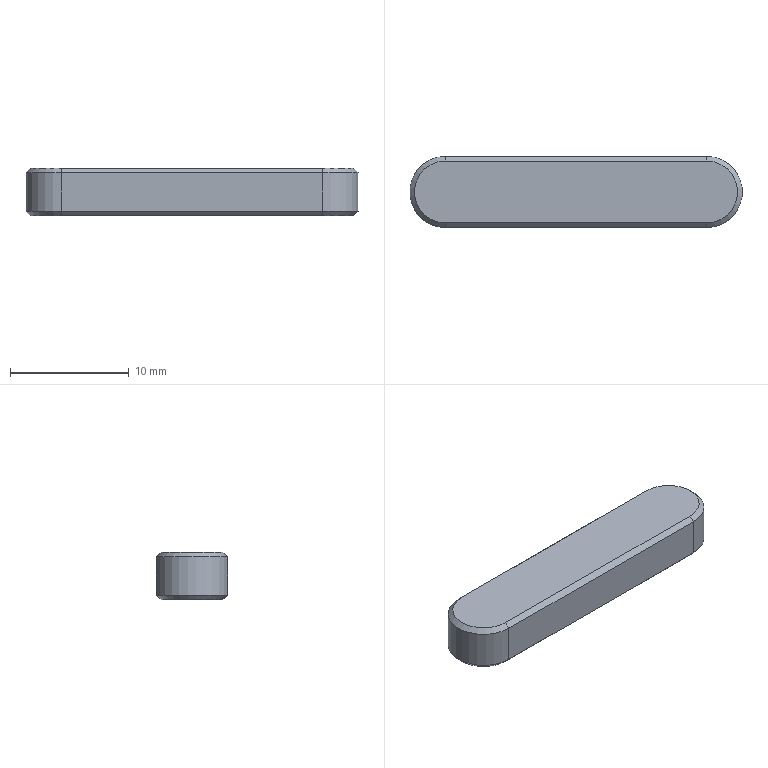Part | SolidWorks | features BaseBody 1 | 1 solid | 14 faces | box 28 x 6 x 4 mm | volume 631.175 mm3 | plane 8 | cone 4 | cylinder 2 | commonest cylinder face diameters 6 x2
STEP:
#1=CARTESIAN_POINT('',(25.,-2.6,-2.5));
#2=VERTEX_POINT('',#1);
#3=CARTESIAN_POINT('',(25.,-3.,-2.1));
#4=VERTEX_POINT('',#3);
#5=CARTESIAN_POINT('',(25.,-2.6,-2.5));
#6=DIRECTION('',(0.,-0.7071,0.7071));
#7=VECTOR('',#6,1000.);
#8=LINE('',#5,#7);
#9=EDGE_CURVE('',#2,#4,#8,.T.);
#10=ORIENTED_EDGE('',*,*,#9,.T.);
#11=CARTESIAN_POINT('',(3.,-3.,-2.1));
#12=VERTEX_POINT('',#11);
#13=CARTESIAN_POINT('',(8.5,-3.,-2.1));
#14=DIRECTION('',(-1.,0.,0.));
#15=VECTOR('',#14,1000.);
#16=LINE('',#13,#15);
#17=EDGE_CURVE('',#4,#12,#16,.T.);
#18=ORIENTED_EDGE('',*,*,#17,.T.);
#19=CARTESIAN_POINT('',(3.,-2.6,-2.5));
#20=VERTEX_POINT('',#19);
#21=CARTESIAN_POINT('',(3.,-3.,-2.1));
#22=DIRECTION('',(0.,0.7071,-0.7071));
#23=VECTOR('',#22,1000.);
#24=LINE('',#21,#23);
#25=EDGE_CURVE('',#12,#20,#24,.T.);
#26=ORIENTED_EDGE('',*,*,#25,.T.);
#27=CARTESIAN_POINT('',(8.5,-2.6,-2.5));
#28=DIRECTION('',(1.,0.,0.));
#29=VECTOR('',#28,1000.);
#30=LINE('',#27,#29);
#31=EDGE_CURVE('',#20,#2,#30,.T.);
#32=ORIENTED_EDGE('',*,*,#31,.T.);
#33=EDGE_LOOP('',(#10,#18,#26,#32));
#34=FACE_OUTER_BOUND('',#33,.T.);
#35=CARTESIAN_POINT('',(8.5,-2.8,-2.3));
#36=DIRECTION('',(0.,-0.7071,-0.7071));
#37=DIRECTION('',(0.,-0.7071,0.7071));
#38=AXIS2_PLACEMENT_3D('',#35,#36,#37);
#39=PLANE('',#38);
#40=ADVANCED_FACE('',(#34),#39,.T.);
#41=CARTESIAN_POINT('',(25.,2.6,-2.5));
#42=VERTEX_POINT('',#41);
#43=CARTESIAN_POINT('',(25.,3.,-2.1));
#44=VERTEX_POINT('',#43);
#45=CARTESIAN_POINT('',(25.,2.6,-2.5));
#46=DIRECTION('',(0.,0.7071,0.7071));
#47=VECTOR('',#46,1000.);
#48=LINE('',#45,#47);
#49=EDGE_CURVE('',#42,#44,#48,.T.);
#50=ORIENTED_EDGE('',*,*,#49,.T.);
#51=CARTESIAN_POINT('',(25.,0.,-2.1));
#52=DIRECTION('',(0.,0.,-1.));
#53=DIRECTION('',(0.,1.,0.));
#54=AXIS2_PLACEMENT_3D('',#51,#52,#53);
#55=CIRCLE('',#54,3.);
#56=EDGE_CURVE('',#44,#4,#55,.T.);
#57=ORIENTED_EDGE('',*,*,#56,.T.);
#58=ORIENTED_EDGE('',*,*,#9,.F.);
#59=CARTESIAN_POINT('',(25.,0.,-2.5));
#60=DIRECTION('',(0.,0.,1.));
#61=DIRECTION('',(0.,1.,0.));
#62=AXIS2_PLACEMENT_3D('',#59,#60,#61);
#63=CIRCLE('',#62,2.6);
#64=EDGE_CURVE('',#2,#42,#63,.T.);
#65=ORIENTED_EDGE('',*,*,#64,.T.);
#66=EDGE_LOOP('',(#50,#57,#58,#65));
#67=FACE_OUTER_BOUND('',#66,.T.);
#68=CARTESIAN_POINT('',(25.,0.,-2.3));
#69=DIRECTION('',(0.,0.,1.));
#70=DIRECTION('',(0.,1.,0.));
#71=AXIS2_PLACEMENT_3D('',#68,#69,#70);
#72=CONICAL_SURFACE('',#71,2.8,0.7854);
#73=ADVANCED_FACE('',(#67),#72,.T.);
#74=CARTESIAN_POINT('',(3.,3.,-2.1));
#75=VERTEX_POINT('',#74);
#76=CARTESIAN_POINT('',(3.,2.6,-2.5));
#77=VERTEX_POINT('',#76);
#78=CARTESIAN_POINT('',(3.,3.,-2.1));
#79=DIRECTION('',(0.,-0.7071,-0.7071));
#80=VECTOR('',#79,1000.);
#81=LINE('',#78,#80);
#82=EDGE_CURVE('',#75,#77,#81,.T.);
#83=ORIENTED_EDGE('',*,*,#82,.T.);
#84=CARTESIAN_POINT('',(3.,0.,-2.5));
#85=DIRECTION('',(0.,0.,1.));
#86=DIRECTION('',(0.,-1.,0.));
#87=AXIS2_PLACEMENT_3D('',#84,#85,#86);
#88=CIRCLE('',#87,2.6);
#89=EDGE_CURVE('',#77,#20,#88,.T.);
#90=ORIENTED_EDGE('',*,*,#89,.T.);
#91=ORIENTED_EDGE('',*,*,#25,.F.);
#92=CARTESIAN_POINT('',(3.,0.,-2.1));
#93=DIRECTION('',(0.,0.,-1.));
#94=DIRECTION('',(0.,-1.,0.));
#95=AXIS2_PLACEMENT_3D('',#92,#93,#94);
#96=CIRCLE('',#95,3.);
#97=EDGE_CURVE('',#12,#75,#96,.T.);
#98=ORIENTED_EDGE('',*,*,#97,.T.);
#99=EDGE_LOOP('',(#83,#90,#91,#98));
#100=FACE_OUTER_BOUND('',#99,.T.);
#101=CARTESIAN_POINT('',(3.,0.,-2.3));
#102=DIRECTION('',(0.,0.,1.));
#103=DIRECTION('',(0.,-1.,0.));
#104=AXIS2_PLACEMENT_3D('',#101,#102,#103);
#105=CONICAL_SURFACE('',#104,2.8,0.7854);
#106=ADVANCED_FACE('',(#100),#105,.T.);
#107=ORIENTED_EDGE('',*,*,#49,.F.);
#108=CARTESIAN_POINT('',(19.5,2.6,-2.5));
#109=DIRECTION('',(-1.,0.,0.));
#110=VECTOR('',#109,1000.);
#111=LINE('',#108,#110);
#112=EDGE_CURVE('',#42,#77,#111,.T.);
#113=ORIENTED_EDGE('',*,*,#112,.T.);
#114=ORIENTED_EDGE('',*,*,#82,.F.);
#115=CARTESIAN_POINT('',(19.5,3.,-2.1));
#116=DIRECTION('',(1.,0.,0.));
#117=VECTOR('',#116,1000.);
#118=LINE('',#115,#117);
#119=EDGE_CURVE('',#75,#44,#118,.T.);
#120=ORIENTED_EDGE('',*,*,#119,.T.);
#121=EDGE_LOOP('',(#107,#113,#114,#120));
#122=FACE_OUTER_BOUND('',#121,.T.);
#123=CARTESIAN_POINT('',(19.5,2.8,-2.3));
#124=DIRECTION('',(0.,0.7071,-0.7071));
#125=DIRECTION('',(-1.,0.,0.));
#126=AXIS2_PLACEMENT_3D('',#123,#124,#125);
#127=PLANE('',#126);
#128=ADVANCED_FACE('',(#122),#127,.T.);
#129=ORIENTED_EDGE('',*,*,#97,.F.);
#130=CARTESIAN_POINT('',(3.,-3.,1.1));
#131=VERTEX_POINT('',#130);
#132=CARTESIAN_POINT('',(3.,-3.,0.));
#133=DIRECTION('',(0.,0.,-1.));
#134=VECTOR('',#133,1000.);
#135=LINE('',#132,#134);
#136=EDGE_CURVE('',#131,#12,#135,.T.);
#137=ORIENTED_EDGE('',*,*,#136,.F.);
#138=CARTESIAN_POINT('',(3.,3.,1.1));
#139=VERTEX_POINT('',#138);
#140=CARTESIAN_POINT('',(3.,0.,1.1));
#141=DIRECTION('',(0.,0.,1.));
#142=DIRECTION('',(0.,-1.,0.));
#143=AXIS2_PLACEMENT_3D('',#140,#141,#142);
#144=CIRCLE('',#143,3.);
#145=EDGE_CURVE('',#139,#131,#144,.T.);
#146=ORIENTED_EDGE('',*,*,#145,.F.);
#147=CARTESIAN_POINT('',(3.,3.,0.));
#148=DIRECTION('',(0.,0.,1.));
#149=VECTOR('',#148,1000.);
#150=LINE('',#147,#149);
#151=EDGE_CURVE('',#75,#139,#150,.T.);
#152=ORIENTED_EDGE('',*,*,#151,.F.);
#153=EDGE_LOOP('',(#129,#137,#146,#152));
#154=FACE_OUTER_BOUND('',#153,.T.);
#155=CARTESIAN_POINT('',(3.,0.,0.));
#156=DIRECTION('',(0.,0.,1.));
#157=DIRECTION('',(0.,-1.,0.));
#158=AXIS2_PLACEMENT_3D('',#155,#156,#157);
#159=CYLINDRICAL_SURFACE('',#158,3.);
#160=ADVANCED_FACE('',(#154),#159,.T.);
#161=ORIENTED_EDGE('',*,*,#17,.F.);
#162=CARTESIAN_POINT('',(25.,-3.,1.1));
#163=VERTEX_POINT('',#162);
#164=CARTESIAN_POINT('',(25.,-3.,0.));
#165=DIRECTION('',(0.,0.,-1.));
#166=VECTOR('',#165,1000.);
#167=LINE('',#164,#166);
#168=EDGE_CURVE('',#163,#4,#167,.T.);
#169=ORIENTED_EDGE('',*,*,#168,.F.);
#170=CARTESIAN_POINT('',(8.5,-3.,1.1));
#171=DIRECTION('',(1.,0.,0.));
#172=VECTOR('',#171,1000.);
#173=LINE('',#170,#172);
#174=EDGE_CURVE('',#131,#163,#173,.T.);
#175=ORIENTED_EDGE('',*,*,#174,.F.);
#176=ORIENTED_EDGE('',*,*,#136,.T.);
#177=EDGE_LOOP('',(#161,#169,#175,#176));
#178=FACE_OUTER_BOUND('',#177,.T.);
#179=CARTESIAN_POINT('',(3.,-3.,0.));
#180=DIRECTION('',(0.,-1.,0.));
#181=DIRECTION('',(0.,0.,-1.));
#182=AXIS2_PLACEMENT_3D('',#179,#180,#181);
#183=PLANE('',#182);
#184=ADVANCED_FACE('',(#178),#183,.T.);
#185=ORIENTED_EDGE('',*,*,#31,.F.);
#186=ORIENTED_EDGE('',*,*,#89,.F.);
#187=ORIENTED_EDGE('',*,*,#112,.F.);
#188=ORIENTED_EDGE('',*,*,#64,.F.);
#189=EDGE_LOOP('',(#185,#186,#187,#188));
#190=FACE_OUTER_BOUND('',#189,.T.);
#191=CARTESIAN_POINT('',(14.,0.,-2.5));
#192=DIRECTION('',(0.,0.,1.));
#193=DIRECTION('',(1.,0.,0.));
#194=AXIS2_PLACEMENT_3D('',#191,#192,#193);
#195=PLANE('',#194);
#196=ADVANCED_FACE('',(#190),#195,.F.);
#197=CARTESIAN_POINT('',(3.,-2.6,1.5));
#198=VERTEX_POINT('',#197);
#199=CARTESIAN_POINT('',(3.,-3.,1.1));
#200=DIRECTION('',(0.,0.7071,0.7071));
#201=VECTOR('',#200,1000.);
#202=LINE('',#199,#201);
#203=EDGE_CURVE('',#131,#198,#202,.T.);
#204=ORIENTED_EDGE('',*,*,#203,.T.);
#205=CARTESIAN_POINT('',(3.,2.6,1.5));
#206=VERTEX_POINT('',#205);
#207=CARTESIAN_POINT('',(3.,0.,1.5));
#208=DIRECTION('',(0.,0.,-1.));
#209=DIRECTION('',(0.,-1.,0.));
#210=AXIS2_PLACEMENT_3D('',#207,#208,#209);
#211=CIRCLE('',#210,2.6);
#212=EDGE_CURVE('',#198,#206,#211,.T.);
#213=ORIENTED_EDGE('',*,*,#212,.T.);
#214=CARTESIAN_POINT('',(3.,2.6,1.5));
#215=DIRECTION('',(0.,0.7071,-0.7071));
#216=VECTOR('',#215,1000.);
#217=LINE('',#214,#216);
#218=EDGE_CURVE('',#206,#139,#217,.T.);
#219=ORIENTED_EDGE('',*,*,#218,.T.);
#220=ORIENTED_EDGE('',*,*,#145,.T.);
#221=EDGE_LOOP('',(#204,#213,#219,#220));
#222=FACE_OUTER_BOUND('',#221,.T.);
#223=CARTESIAN_POINT('',(3.,0.,1.3));
#224=DIRECTION('',(0.,0.,-1.));
#225=DIRECTION('',(0.,-1.,0.));
#226=AXIS2_PLACEMENT_3D('',#223,#224,#225);
#227=CONICAL_SURFACE('',#226,2.8,0.7854);
#228=ADVANCED_FACE('',(#222),#227,.T.);
#229=CARTESIAN_POINT('',(25.,-2.6,1.5));
#230=VERTEX_POINT('',#229);
#231=CARTESIAN_POINT('',(25.,-3.,1.1));
#232=DIRECTION('',(0.,0.7071,0.7071));
#233=VECTOR('',#232,1000.);
#234=LINE('',#231,#233);
#235=EDGE_CURVE('',#163,#230,#234,.T.);
#236=ORIENTED_EDGE('',*,*,#235,.T.);
#237=CARTESIAN_POINT('',(8.5,-2.6,1.5));
#238=DIRECTION('',(-1.,0.,0.));
#239=VECTOR('',#238,1000.);
#240=LINE('',#237,#239);
#241=EDGE_CURVE('',#230,#198,#240,.T.);
#242=ORIENTED_EDGE('',*,*,#241,.T.);
#243=ORIENTED_EDGE('',*,*,#203,.F.);
#244=ORIENTED_EDGE('',*,*,#174,.T.);
#245=EDGE_LOOP('',(#236,#242,#243,#244));
#246=FACE_OUTER_BOUND('',#245,.T.);
#247=CARTESIAN_POINT('',(8.5,-2.8,1.3));
#248=DIRECTION('',(0.,-0.7071,0.7071));
#249=DIRECTION('',(-1.,0.,0.));
#250=AXIS2_PLACEMENT_3D('',#247,#248,#249);
#251=PLANE('',#250);
#252=ADVANCED_FACE('',(#246),#251,.T.);
#253=CARTESIAN_POINT('',(25.,2.6,1.5));
#254=VERTEX_POINT('',#253);
#255=CARTESIAN_POINT('',(25.,3.,1.1));
#256=VERTEX_POINT('',#255);
#257=CARTESIAN_POINT('',(25.,2.6,1.5));
#258=DIRECTION('',(0.,0.7071,-0.7071));
#259=VECTOR('',#258,1000.);
#260=LINE('',#257,#259);
#261=EDGE_CURVE('',#254,#256,#260,.T.);
#262=ORIENTED_EDGE('',*,*,#261,.T.);
#263=CARTESIAN_POINT('',(19.5,3.,1.1));
#264=DIRECTION('',(-1.,0.,0.));
#265=VECTOR('',#264,1000.);
#266=LINE('',#263,#265);
#267=EDGE_CURVE('',#256,#139,#266,.T.);
#268=ORIENTED_EDGE('',*,*,#267,.T.);
#269=ORIENTED_EDGE('',*,*,#218,.F.);
#270=CARTESIAN_POINT('',(19.5,2.6,1.5));
#271=DIRECTION('',(1.,0.,0.));
#272=VECTOR('',#271,1000.);
#273=LINE('',#270,#272);
#274=EDGE_CURVE('',#206,#254,#273,.T.);
#275=ORIENTED_EDGE('',*,*,#274,.T.);
#276=EDGE_LOOP('',(#262,#268,#269,#275));
#277=FACE_OUTER_BOUND('',#276,.T.);
#278=CARTESIAN_POINT('',(19.5,2.8,1.3));
#279=DIRECTION('',(0.,0.7071,0.7071));
#280=DIRECTION('',(1.,0.,0.));
#281=AXIS2_PLACEMENT_3D('',#278,#279,#280);
#282=PLANE('',#281);
#283=ADVANCED_FACE('',(#277),#282,.T.);
#284=ORIENTED_EDGE('',*,*,#235,.F.);
#285=CARTESIAN_POINT('',(25.,0.,1.1));
#286=DIRECTION('',(0.,0.,1.));
#287=DIRECTION('',(0.,1.,0.));
#288=AXIS2_PLACEMENT_3D('',#285,#286,#287);
#289=CIRCLE('',#288,3.);
#290=EDGE_CURVE('',#163,#256,#289,.T.);
#291=ORIENTED_EDGE('',*,*,#290,.T.);
#292=ORIENTED_EDGE('',*,*,#261,.F.);
#293=CARTESIAN_POINT('',(25.,0.,1.5));
#294=DIRECTION('',(0.,0.,-1.));
#295=DIRECTION('',(0.,1.,0.));
#296=AXIS2_PLACEMENT_3D('',#293,#294,#295);
#297=CIRCLE('',#296,2.6);
#298=EDGE_CURVE('',#254,#230,#297,.T.);
#299=ORIENTED_EDGE('',*,*,#298,.T.);
#300=EDGE_LOOP('',(#284,#291,#292,#299));
#301=FACE_OUTER_BOUND('',#300,.T.);
#302=CARTESIAN_POINT('',(25.,0.,1.3));
#303=DIRECTION('',(0.,0.,-1.));
#304=DIRECTION('',(0.,1.,0.));
#305=AXIS2_PLACEMENT_3D('',#302,#303,#304);
#306=CONICAL_SURFACE('',#305,2.8,0.7854);
#307=ADVANCED_FACE('',(#301),#306,.T.);
#308=ORIENTED_EDGE('',*,*,#212,.F.);
#309=ORIENTED_EDGE('',*,*,#241,.F.);
#310=ORIENTED_EDGE('',*,*,#298,.F.);
#311=ORIENTED_EDGE('',*,*,#274,.F.);
#312=EDGE_LOOP('',(#308,#309,#310,#311));
#313=FACE_OUTER_BOUND('',#312,.T.);
#314=CARTESIAN_POINT('',(14.,0.,1.5));
#315=DIRECTION('',(0.,0.,1.));
#316=DIRECTION('',(1.,0.,0.));
#317=AXIS2_PLACEMENT_3D('',#314,#315,#316);
#318=PLANE('',#317);
#319=ADVANCED_FACE('',(#313),#318,.T.);
#320=ORIENTED_EDGE('',*,*,#119,.F.);
#321=ORIENTED_EDGE('',*,*,#151,.T.);
#322=ORIENTED_EDGE('',*,*,#267,.F.);
#323=CARTESIAN_POINT('',(25.,3.,0.));
#324=DIRECTION('',(0.,0.,-1.));
#325=VECTOR('',#324,1000.);
#326=LINE('',#323,#325);
#327=EDGE_CURVE('',#256,#44,#326,.T.);
#328=ORIENTED_EDGE('',*,*,#327,.T.);
#329=EDGE_LOOP('',(#320,#321,#322,#328));
#330=FACE_OUTER_BOUND('',#329,.T.);
#331=CARTESIAN_POINT('',(25.,3.,0.));
#332=DIRECTION('',(0.,1.,0.));
#333=DIRECTION('',(1.,0.,0.));
#334=AXIS2_PLACEMENT_3D('',#331,#332,#333);
#335=PLANE('',#334);
#336=ADVANCED_FACE('',(#330),#335,.T.);
#337=ORIENTED_EDGE('',*,*,#56,.F.);
#338=ORIENTED_EDGE('',*,*,#327,.F.);
#339=ORIENTED_EDGE('',*,*,#290,.F.);
#340=ORIENTED_EDGE('',*,*,#168,.T.);
#341=EDGE_LOOP('',(#337,#338,#339,#340));
#342=FACE_OUTER_BOUND('',#341,.T.);
#343=CARTESIAN_POINT('',(25.,0.,0.));
#344=DIRECTION('',(0.,0.,1.));
#345=DIRECTION('',(0.,1.,0.));
#346=AXIS2_PLACEMENT_3D('',#343,#344,#345);
#347=CYLINDRICAL_SURFACE('',#346,3.);
#348=ADVANCED_FACE('',(#342),#347,.T.);
#349=CLOSED_SHELL('',(#40,#73,#106,#128,#160,#184,#196,#228,#252,#283,#307,#319,#336,#348));
#350=MANIFOLD_SOLID_BREP('',#349);
#351=CARTESIAN_POINT('',(0.,0.,0.));
#352=DIRECTION('',(0.,0.,1.));
#353=DIRECTION('',(1.,0.,0.));
#354=AXIS2_PLACEMENT_3D('',#351,#352,#353);
#355=(LENGTH_UNIT()NAMED_UNIT(*)SI_UNIT(.MILLI.,.METRE.));
#356=UNCERTAINTY_MEASURE_WITH_UNIT(LENGTH_MEASURE(0.00001),#355,'','');
#357=(NAMED_UNIT(*)PLANE_ANGLE_UNIT()SI_UNIT($,.RADIAN.));
#358=(NAMED_UNIT(*)SI_UNIT($,.STERADIAN.)SOLID_ANGLE_UNIT());
#359=(GEOMETRIC_REPRESENTATION_CONTEXT(3)GLOBAL_UNCERTAINTY_ASSIGNED_CONTEXT((#356))GLOBAL_UNIT_ASSIGNED_CONTEXT((#355,#357,#358))REPRESENTATION_CONTEXT('',''));
#360=ADVANCED_BREP_SHAPE_REPRESENTATION('',(#350,#354),#359);